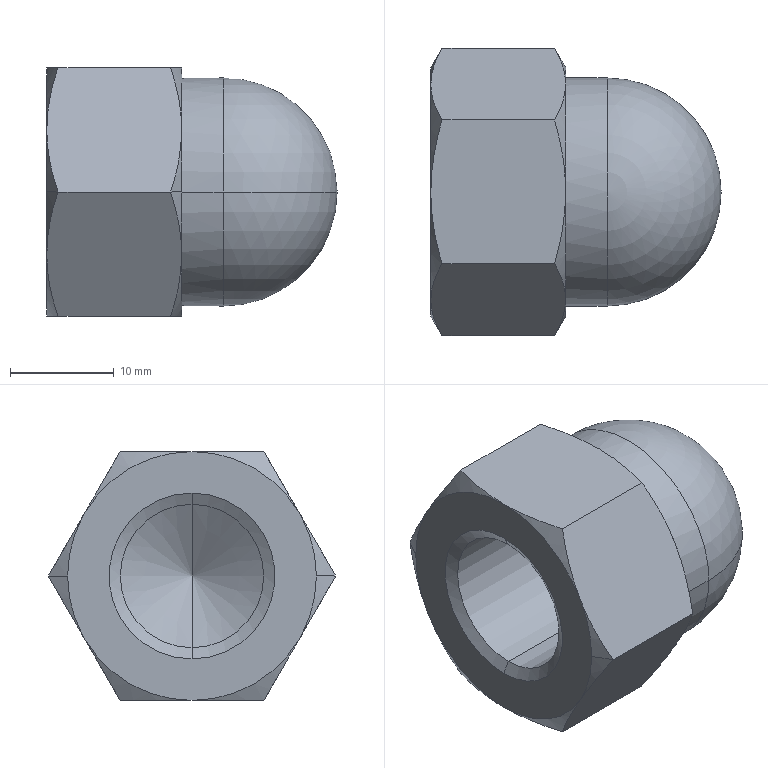Part | STEP file | KS B 1026 Type 1 - M16 | 1 solid | 34 faces | box 28 x 27.713 x 24 mm | volume 8094 mm3 | cone 20 | plane 8 | cylinder 4 | sphere 2 | commonest cylinder face diameters 13.835 x2 22 x2